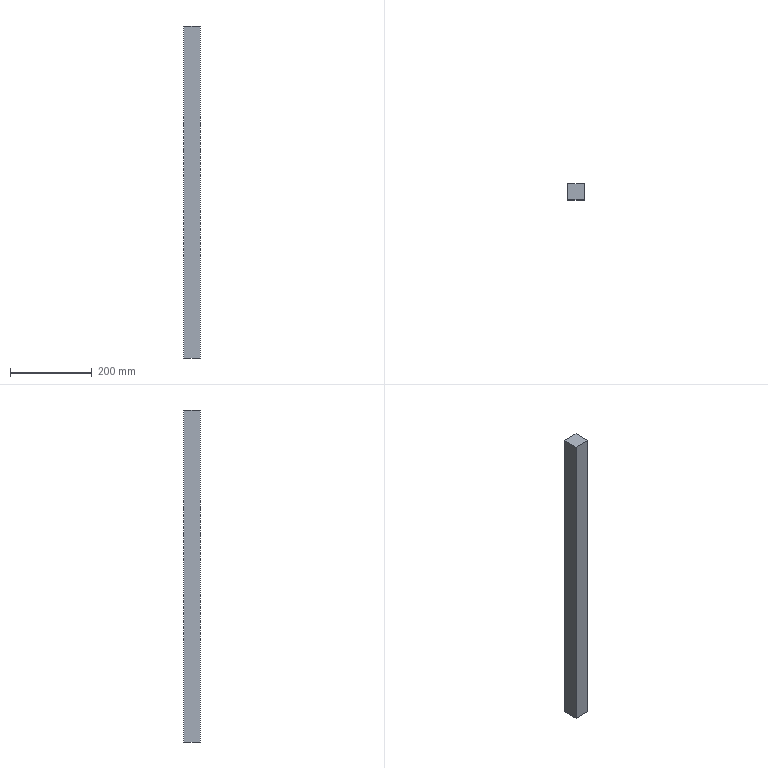Part | NX | features 凸台-拉伸24 2 | 1 solid | 6 faces | box 40 x 40 x 810 mm | volume 1296000 mm3 | plane 6
STEP:
#1=CARTESIAN_POINT('',(1823.,-560.,-1062.985));
#2=VERTEX_POINT('',#1);
#3=CARTESIAN_POINT('',(1863.,-560.,-1062.985));
#4=VERTEX_POINT('',#3);
#5=CARTESIAN_POINT('',(1863.,-560.,-1062.985));
#6=DIRECTION('',(1.,0.,0.));
#7=VECTOR('',#6,1000.);
#8=LINE('',#5,#7);
#9=EDGE_CURVE('',#2,#4,#8,.T.);
#10=ORIENTED_EDGE('',*,*,#9,.T.);
#11=CARTESIAN_POINT('',(1863.,-600.,-1062.985));
#12=VERTEX_POINT('',#11);
#13=CARTESIAN_POINT('',(1863.,-600.,-1062.985));
#14=DIRECTION('',(0.,-1.,0.));
#15=VECTOR('',#14,1000.);
#16=LINE('',#13,#15);
#17=EDGE_CURVE('',#4,#12,#16,.T.);
#18=ORIENTED_EDGE('',*,*,#17,.T.);
#19=CARTESIAN_POINT('',(1823.,-600.,-1062.985));
#20=VERTEX_POINT('',#19);
#21=CARTESIAN_POINT('',(1863.,-600.,-1062.985));
#22=DIRECTION('',(-1.,0.,0.));
#23=VECTOR('',#22,1000.);
#24=LINE('',#21,#23);
#25=EDGE_CURVE('',#12,#20,#24,.T.);
#26=ORIENTED_EDGE('',*,*,#25,.T.);
#27=CARTESIAN_POINT('',(1823.,-600.,-1062.985));
#28=DIRECTION('',(0.,1.,0.));
#29=VECTOR('',#28,1000.);
#30=LINE('',#27,#29);
#31=EDGE_CURVE('',#20,#2,#30,.T.);
#32=ORIENTED_EDGE('',*,*,#31,.T.);
#33=EDGE_LOOP('',(#10,#18,#26,#32));
#34=FACE_BOUND('',#33,.T.);
#35=CARTESIAN_POINT('',(2849.569,-560.,-1062.985));
#36=DIRECTION('',(0.,0.,-1.));
#37=DIRECTION('',(-1.,0.,0.));
#38=AXIS2_PLACEMENT_3D('',#35,#36,#37);
#39=PLANE('',#38);
#40=ADVANCED_FACE('',(#34),#39,.T.);
#41=CARTESIAN_POINT('',(1863.,-560.,-252.985));
#42=VERTEX_POINT('',#41);
#43=CARTESIAN_POINT('',(1863.,-600.,-252.985));
#44=VERTEX_POINT('',#43);
#45=CARTESIAN_POINT('',(1863.,-600.,-252.985));
#46=DIRECTION('',(0.,-1.,0.));
#47=VECTOR('',#46,1000.);
#48=LINE('',#45,#47);
#49=EDGE_CURVE('',#42,#44,#48,.T.);
#50=ORIENTED_EDGE('',*,*,#49,.F.);
#51=CARTESIAN_POINT('',(1823.,-560.,-252.985));
#52=VERTEX_POINT('',#51);
#53=CARTESIAN_POINT('',(1863.,-560.,-252.985));
#54=DIRECTION('',(1.,0.,0.));
#55=VECTOR('',#54,1000.);
#56=LINE('',#53,#55);
#57=EDGE_CURVE('',#52,#42,#56,.T.);
#58=ORIENTED_EDGE('',*,*,#57,.F.);
#59=CARTESIAN_POINT('',(1823.,-600.,-252.985));
#60=VERTEX_POINT('',#59);
#61=CARTESIAN_POINT('',(1823.,-600.,-252.985));
#62=DIRECTION('',(0.,1.,0.));
#63=VECTOR('',#62,1000.);
#64=LINE('',#61,#63);
#65=EDGE_CURVE('',#60,#52,#64,.T.);
#66=ORIENTED_EDGE('',*,*,#65,.F.);
#67=CARTESIAN_POINT('',(1863.,-600.,-252.985));
#68=DIRECTION('',(-1.,0.,0.));
#69=VECTOR('',#68,1000.);
#70=LINE('',#67,#69);
#71=EDGE_CURVE('',#44,#60,#70,.T.);
#72=ORIENTED_EDGE('',*,*,#71,.F.);
#73=EDGE_LOOP('',(#50,#58,#66,#72));
#74=FACE_BOUND('',#73,.T.);
#75=CARTESIAN_POINT('',(1500.,0.,-252.985));
#76=DIRECTION('',(0.,0.,1.));
#77=DIRECTION('',(1.,0.,0.));
#78=AXIS2_PLACEMENT_3D('',#75,#76,#77);
#79=PLANE('',#78);
#80=ADVANCED_FACE('',(#74),#79,.T.);
#81=ORIENTED_EDGE('',*,*,#9,.F.);
#82=CARTESIAN_POINT('',(1823.,-560.,-1119.553));
#83=DIRECTION('',(0.,0.,1.));
#84=VECTOR('',#83,1000.);
#85=LINE('',#82,#84);
#86=EDGE_CURVE('',#2,#52,#85,.T.);
#87=ORIENTED_EDGE('',*,*,#86,.T.);
#88=ORIENTED_EDGE('',*,*,#57,.T.);
#89=CARTESIAN_POINT('',(1863.,-560.,-1119.553));
#90=DIRECTION('',(0.,0.,1.));
#91=VECTOR('',#90,1000.);
#92=LINE('',#89,#91);
#93=EDGE_CURVE('',#4,#42,#92,.T.);
#94=ORIENTED_EDGE('',*,*,#93,.F.);
#95=EDGE_LOOP('',(#81,#87,#88,#94));
#96=FACE_BOUND('',#95,.T.);
#97=CARTESIAN_POINT('',(1863.,-560.,-1119.553));
#98=DIRECTION('',(0.,-1.,0.));
#99=DIRECTION('',(0.,0.,-1.));
#100=AXIS2_PLACEMENT_3D('',#97,#98,#99);
#101=PLANE('',#100);
#102=ADVANCED_FACE('',(#96),#101,.F.);
#103=ORIENTED_EDGE('',*,*,#31,.F.);
#104=CARTESIAN_POINT('',(1823.,-600.,-1119.553));
#105=DIRECTION('',(0.,0.,1.));
#106=VECTOR('',#105,1000.);
#107=LINE('',#104,#106);
#108=EDGE_CURVE('',#20,#60,#107,.T.);
#109=ORIENTED_EDGE('',*,*,#108,.T.);
#110=ORIENTED_EDGE('',*,*,#65,.T.);
#111=ORIENTED_EDGE('',*,*,#86,.F.);
#112=EDGE_LOOP('',(#103,#109,#110,#111));
#113=FACE_BOUND('',#112,.T.);
#114=CARTESIAN_POINT('',(1823.,-600.,-1119.553));
#115=DIRECTION('',(1.,0.,0.));
#116=DIRECTION('',(0.,0.,-1.));
#117=AXIS2_PLACEMENT_3D('',#114,#115,#116);
#118=PLANE('',#117);
#119=ADVANCED_FACE('',(#113),#118,.F.);
#120=ORIENTED_EDGE('',*,*,#25,.F.);
#121=CARTESIAN_POINT('',(1863.,-600.,-1119.553));
#122=DIRECTION('',(0.,0.,1.));
#123=VECTOR('',#122,1000.);
#124=LINE('',#121,#123);
#125=EDGE_CURVE('',#12,#44,#124,.T.);
#126=ORIENTED_EDGE('',*,*,#125,.T.);
#127=ORIENTED_EDGE('',*,*,#71,.T.);
#128=ORIENTED_EDGE('',*,*,#108,.F.);
#129=EDGE_LOOP('',(#120,#126,#127,#128));
#130=FACE_BOUND('',#129,.T.);
#131=CARTESIAN_POINT('',(1863.,-600.,-1119.553));
#132=DIRECTION('',(0.,1.,0.));
#133=DIRECTION('',(0.,0.,1.));
#134=AXIS2_PLACEMENT_3D('',#131,#132,#133);
#135=PLANE('',#134);
#136=ADVANCED_FACE('',(#130),#135,.F.);
#137=ORIENTED_EDGE('',*,*,#17,.F.);
#138=ORIENTED_EDGE('',*,*,#93,.T.);
#139=ORIENTED_EDGE('',*,*,#49,.T.);
#140=ORIENTED_EDGE('',*,*,#125,.F.);
#141=EDGE_LOOP('',(#137,#138,#139,#140));
#142=FACE_BOUND('',#141,.T.);
#143=CARTESIAN_POINT('',(1863.,-600.,-1119.553));
#144=DIRECTION('',(-1.,0.,0.));
#145=DIRECTION('',(0.,0.,1.));
#146=AXIS2_PLACEMENT_3D('',#143,#144,#145);
#147=PLANE('',#146);
#148=ADVANCED_FACE('',(#142),#147,.F.);
#149=CLOSED_SHELL('',(#40,#80,#102,#119,#136,#148));
#150=MANIFOLD_SOLID_BREP('',#149);
#151=(LENGTH_UNIT()NAMED_UNIT(*)SI_UNIT(.MILLI.,.METRE.));
#152=UNCERTAINTY_MEASURE_WITH_UNIT(LENGTH_MEASURE(0.00001),#151,'','');
#153=(NAMED_UNIT(*)PLANE_ANGLE_UNIT()SI_UNIT($,.RADIAN.));
#154=(NAMED_UNIT(*)SI_UNIT($,.STERADIAN.)SOLID_ANGLE_UNIT());
#155=(GEOMETRIC_REPRESENTATION_CONTEXT(3)GLOBAL_UNCERTAINTY_ASSIGNED_CONTEXT((#152))GLOBAL_UNIT_ASSIGNED_CONTEXT((#151,#153,#154))REPRESENTATION_CONTEXT('',''));
#156=ADVANCED_BREP_SHAPE_REPRESENTATION('',(#150),#155);